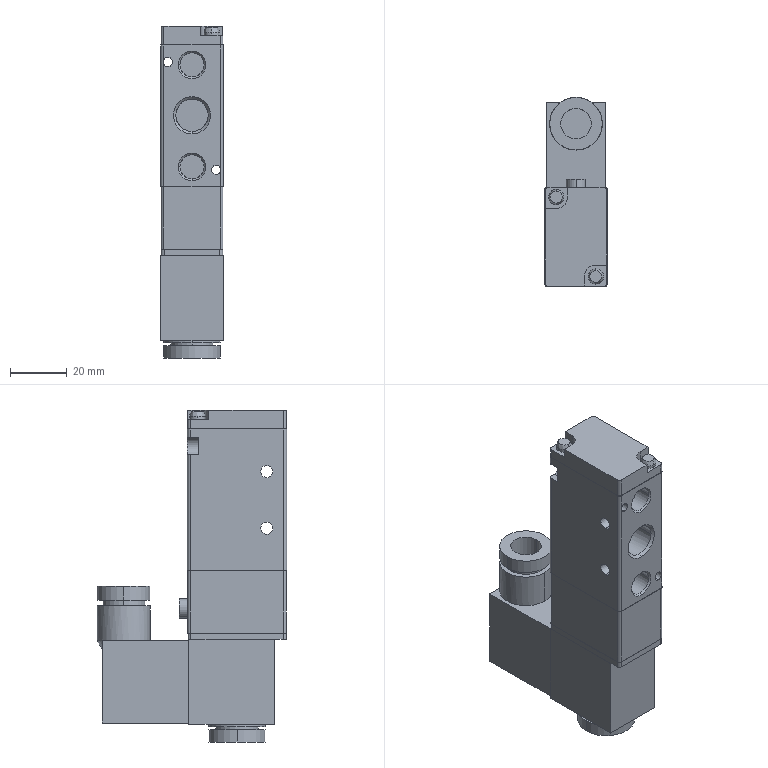Part | SolidWorks | features BaseBody 1 | 1 solid | 138 faces | box 22 x 66.8 x 117.1 mm | volume 99652 mm3 | cylinder 61 | plane 61 | cone 12 | spline 4 | commonest cylinder face diameters 2 x18 11.445 x6 3.2 x4 4.3 x4 5.4 x4 8.566 x4